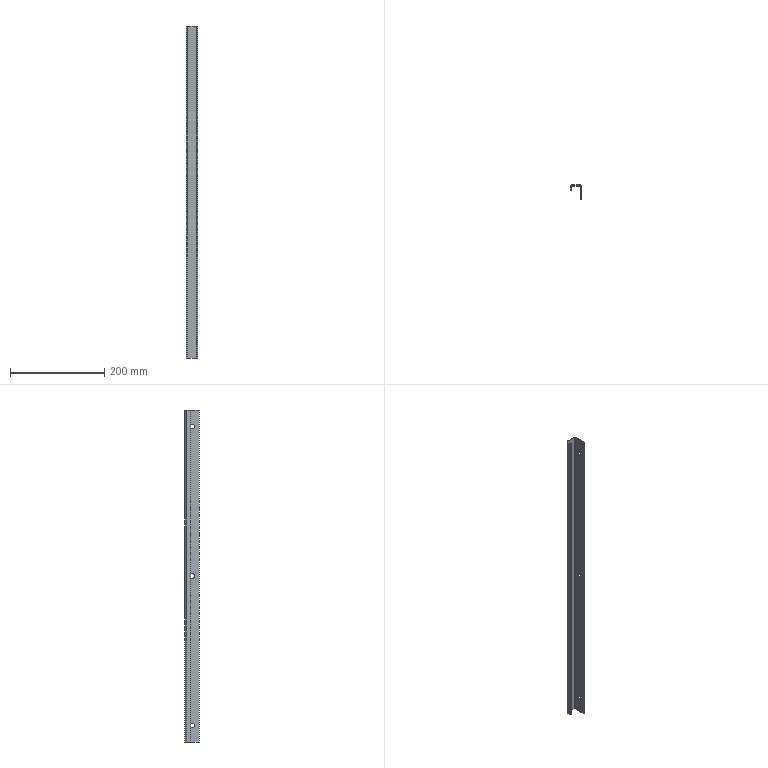Part | STEP file | 750078266 | 1 solid | 20 faces | box 25 x 30 x 704 mm | volume 84559 mm3 | cylinder 10 | plane 10 | commonest cylinder face diameters 10.5 x6 4 x2 8 x2
STEP:
#1=CARTESIAN_POINT('',(-2.,15.,322.25));
#2=VERTEX_POINT('',#1);
#3=CARTESIAN_POINT('',(-2.,15.,311.75));
#4=VERTEX_POINT('',#3);
#5=CARTESIAN_POINT('',(-2.,15.,317.));
#6=DIRECTION('',(1.,0.,0.));
#7=DIRECTION('',(0.,0.,-1.));
#8=AXIS2_PLACEMENT_3D('',#5,#6,#7);
#9=CIRCLE('',#8,5.25);
#10=EDGE_CURVE('',#2,#4,#9,.T.);
#11=ORIENTED_EDGE('',*,*,#10,.F.);
#12=CARTESIAN_POINT('',(0.,15.,322.25));
#13=VERTEX_POINT('',#12);
#14=CARTESIAN_POINT('',(-2.,15.,322.25));
#15=DIRECTION('',(1.,0.,0.));
#16=VECTOR('',#15,1000.);
#17=LINE('',#14,#16);
#18=EDGE_CURVE('',#2,#13,#17,.T.);
#19=ORIENTED_EDGE('',*,*,#18,.T.);
#20=CARTESIAN_POINT('',(0.,15.,311.75));
#21=VERTEX_POINT('',#20);
#22=CARTESIAN_POINT('',(0.,15.,317.));
#23=DIRECTION('',(-1.,0.,0.));
#24=DIRECTION('',(0.,0.,-1.));
#25=AXIS2_PLACEMENT_3D('',#22,#23,#24);
#26=CIRCLE('',#25,5.25);
#27=EDGE_CURVE('',#21,#13,#26,.T.);
#28=ORIENTED_EDGE('',*,*,#27,.F.);
#29=CARTESIAN_POINT('',(-2.,15.,311.75));
#30=DIRECTION('',(1.,0.,0.));
#31=VECTOR('',#30,1000.);
#32=LINE('',#29,#31);
#33=EDGE_CURVE('',#4,#21,#32,.T.);
#34=ORIENTED_EDGE('',*,*,#33,.F.);
#35=EDGE_LOOP('',(#11,#19,#28,#34));
#36=FACE_OUTER_BOUND('',#35,.T.);
#37=CARTESIAN_POINT('',(-2.,15.,317.));
#38=DIRECTION('',(1.,0.,0.));
#39=DIRECTION('',(0.,0.,-1.));
#40=AXIS2_PLACEMENT_3D('',#37,#38,#39);
#41=CYLINDRICAL_SURFACE('',#40,5.25);
#42=ADVANCED_FACE('',(#36),#41,.F.);
#43=CARTESIAN_POINT('',(-2.,15.,5.25));
#44=VERTEX_POINT('',#43);
#45=CARTESIAN_POINT('',(-2.,15.,-5.25));
#46=VERTEX_POINT('',#45);
#47=CARTESIAN_POINT('',(-2.,15.,0.));
#48=DIRECTION('',(1.,0.,0.));
#49=DIRECTION('',(0.,0.,-1.));
#50=AXIS2_PLACEMENT_3D('',#47,#48,#49);
#51=CIRCLE('',#50,5.25);
#52=EDGE_CURVE('',#44,#46,#51,.T.);
#53=ORIENTED_EDGE('',*,*,#52,.F.);
#54=CARTESIAN_POINT('',(0.,15.,5.25));
#55=VERTEX_POINT('',#54);
#56=CARTESIAN_POINT('',(-2.,15.,5.25));
#57=DIRECTION('',(1.,0.,0.));
#58=VECTOR('',#57,1000.);
#59=LINE('',#56,#58);
#60=EDGE_CURVE('',#44,#55,#59,.T.);
#61=ORIENTED_EDGE('',*,*,#60,.T.);
#62=CARTESIAN_POINT('',(0.,15.,-5.25));
#63=VERTEX_POINT('',#62);
#64=CARTESIAN_POINT('',(0.,15.,0.));
#65=DIRECTION('',(-1.,0.,0.));
#66=DIRECTION('',(0.,0.,-1.));
#67=AXIS2_PLACEMENT_3D('',#64,#65,#66);
#68=CIRCLE('',#67,5.25);
#69=EDGE_CURVE('',#63,#55,#68,.T.);
#70=ORIENTED_EDGE('',*,*,#69,.F.);
#71=CARTESIAN_POINT('',(-2.,15.,-5.25));
#72=DIRECTION('',(1.,0.,0.));
#73=VECTOR('',#72,1000.);
#74=LINE('',#71,#73);
#75=EDGE_CURVE('',#46,#63,#74,.T.);
#76=ORIENTED_EDGE('',*,*,#75,.F.);
#77=EDGE_LOOP('',(#53,#61,#70,#76));
#78=FACE_OUTER_BOUND('',#77,.T.);
#79=CARTESIAN_POINT('',(-2.,15.,0.));
#80=DIRECTION('',(1.,0.,0.));
#81=DIRECTION('',(0.,0.,-1.));
#82=AXIS2_PLACEMENT_3D('',#79,#80,#81);
#83=CYLINDRICAL_SURFACE('',#82,5.25);
#84=ADVANCED_FACE('',(#78),#83,.F.);
#85=CARTESIAN_POINT('',(-2.,15.,-311.75));
#86=VERTEX_POINT('',#85);
#87=CARTESIAN_POINT('',(-2.,15.,-322.25));
#88=VERTEX_POINT('',#87);
#89=CARTESIAN_POINT('',(-2.,15.,-317.));
#90=DIRECTION('',(1.,0.,0.));
#91=DIRECTION('',(0.,0.,-1.));
#92=AXIS2_PLACEMENT_3D('',#89,#90,#91);
#93=CIRCLE('',#92,5.25);
#94=EDGE_CURVE('',#86,#88,#93,.T.);
#95=ORIENTED_EDGE('',*,*,#94,.F.);
#96=CARTESIAN_POINT('',(0.,15.,-311.75));
#97=VERTEX_POINT('',#96);
#98=CARTESIAN_POINT('',(-2.,15.,-311.75));
#99=DIRECTION('',(1.,0.,0.));
#100=VECTOR('',#99,1000.);
#101=LINE('',#98,#100);
#102=EDGE_CURVE('',#86,#97,#101,.T.);
#103=ORIENTED_EDGE('',*,*,#102,.T.);
#104=CARTESIAN_POINT('',(0.,15.,-322.25));
#105=VERTEX_POINT('',#104);
#106=CARTESIAN_POINT('',(0.,15.,-317.));
#107=DIRECTION('',(-1.,0.,0.));
#108=DIRECTION('',(0.,0.,-1.));
#109=AXIS2_PLACEMENT_3D('',#106,#107,#108);
#110=CIRCLE('',#109,5.25);
#111=EDGE_CURVE('',#105,#97,#110,.T.);
#112=ORIENTED_EDGE('',*,*,#111,.F.);
#113=CARTESIAN_POINT('',(-2.,15.,-322.25));
#114=DIRECTION('',(1.,0.,0.));
#115=VECTOR('',#114,1000.);
#116=LINE('',#113,#115);
#117=EDGE_CURVE('',#88,#105,#116,.T.);
#118=ORIENTED_EDGE('',*,*,#117,.F.);
#119=EDGE_LOOP('',(#95,#103,#112,#118));
#120=FACE_OUTER_BOUND('',#119,.T.);
#121=CARTESIAN_POINT('',(-2.,15.,-317.));
#122=DIRECTION('',(1.,0.,0.));
#123=DIRECTION('',(0.,0.,-1.));
#124=AXIS2_PLACEMENT_3D('',#121,#122,#123);
#125=CYLINDRICAL_SURFACE('',#124,5.25);
#126=ADVANCED_FACE('',(#120),#125,.F.);
#127=CARTESIAN_POINT('',(0.,26.,352.));
#128=VERTEX_POINT('',#127);
#129=CARTESIAN_POINT('',(0.,0.,352.));
#130=VERTEX_POINT('',#129);
#131=CARTESIAN_POINT('',(0.,30.,352.));
#132=DIRECTION('',(0.,-1.,0.));
#133=VECTOR('',#132,1000.);
#134=LINE('',#131,#133);
#135=EDGE_CURVE('',#128,#130,#134,.T.);
#136=ORIENTED_EDGE('',*,*,#135,.T.);
#137=CARTESIAN_POINT('',(0.,0.,-352.));
#138=VERTEX_POINT('',#137);
#139=CARTESIAN_POINT('',(0.,0.,352.));
#140=DIRECTION('',(0.,0.,-1.));
#141=VECTOR('',#140,1000.);
#142=LINE('',#139,#141);
#143=EDGE_CURVE('',#130,#138,#142,.T.);
#144=ORIENTED_EDGE('',*,*,#143,.T.);
#145=CARTESIAN_POINT('',(0.,26.,-352.));
#146=VERTEX_POINT('',#145);
#147=CARTESIAN_POINT('',(0.,30.,-352.));
#148=DIRECTION('',(0.,1.,0.));
#149=VECTOR('',#148,1000.);
#150=LINE('',#147,#149);
#151=EDGE_CURVE('',#138,#146,#150,.T.);
#152=ORIENTED_EDGE('',*,*,#151,.T.);
#153=CARTESIAN_POINT('',(0.,26.,352.));
#154=DIRECTION('',(0.,0.,1.));
#155=VECTOR('',#154,1000.);
#156=LINE('',#153,#155);
#157=EDGE_CURVE('',#146,#128,#156,.T.);
#158=ORIENTED_EDGE('',*,*,#157,.T.);
#159=EDGE_LOOP('',(#136,#144,#152,#158));
#160=FACE_OUTER_BOUND('',#159,.T.);
#161=ORIENTED_EDGE('',*,*,#27,.T.);
#162=CARTESIAN_POINT('',(0.,15.,317.));
#163=DIRECTION('',(-1.,0.,0.));
#164=DIRECTION('',(0.,0.,-1.));
#165=AXIS2_PLACEMENT_3D('',#162,#163,#164);
#166=CIRCLE('',#165,5.25);
#167=EDGE_CURVE('',#13,#21,#166,.T.);
#168=ORIENTED_EDGE('',*,*,#167,.T.);
#169=EDGE_LOOP('',(#161,#168));
#170=FACE_BOUND('',#169,.T.);
#171=ORIENTED_EDGE('',*,*,#69,.T.);
#172=CARTESIAN_POINT('',(0.,15.,0.));
#173=DIRECTION('',(-1.,0.,0.));
#174=DIRECTION('',(0.,0.,-1.));
#175=AXIS2_PLACEMENT_3D('',#172,#173,#174);
#176=CIRCLE('',#175,5.25);
#177=EDGE_CURVE('',#55,#63,#176,.T.);
#178=ORIENTED_EDGE('',*,*,#177,.T.);
#179=EDGE_LOOP('',(#171,#178));
#180=FACE_BOUND('',#179,.T.);
#181=ORIENTED_EDGE('',*,*,#111,.T.);
#182=CARTESIAN_POINT('',(0.,15.,-317.));
#183=DIRECTION('',(-1.,0.,0.));
#184=DIRECTION('',(0.,0.,-1.));
#185=AXIS2_PLACEMENT_3D('',#182,#183,#184);
#186=CIRCLE('',#185,5.25);
#187=EDGE_CURVE('',#97,#105,#186,.T.);
#188=ORIENTED_EDGE('',*,*,#187,.T.);
#189=EDGE_LOOP('',(#181,#188));
#190=FACE_BOUND('',#189,.T.);
#191=CARTESIAN_POINT('',(0.,30.,352.));
#192=DIRECTION('',(1.,0.,0.));
#193=DIRECTION('',(0.,0.,-1.));
#194=AXIS2_PLACEMENT_3D('',#191,#192,#193);
#195=PLANE('',#194);
#196=ADVANCED_FACE('',(#160,#170,#180,#190),#195,.T.);
#197=CARTESIAN_POINT('',(-2.,0.,-352.));
#198=VERTEX_POINT('',#197);
#199=CARTESIAN_POINT('',(0.,0.,-352.));
#200=DIRECTION('',(1.,0.,0.));
#201=VECTOR('',#200,1000.);
#202=LINE('',#199,#201);
#203=EDGE_CURVE('',#198,#138,#202,.T.);
#204=ORIENTED_EDGE('',*,*,#203,.T.);
#205=ORIENTED_EDGE('',*,*,#143,.F.);
#206=CARTESIAN_POINT('',(-2.,0.,352.));
#207=VERTEX_POINT('',#206);
#208=CARTESIAN_POINT('',(0.,0.,352.));
#209=DIRECTION('',(-1.,0.,0.));
#210=VECTOR('',#209,1000.);
#211=LINE('',#208,#210);
#212=EDGE_CURVE('',#130,#207,#211,.T.);
#213=ORIENTED_EDGE('',*,*,#212,.T.);
#214=CARTESIAN_POINT('',(-2.,0.,352.));
#215=DIRECTION('',(0.,0.,-1.));
#216=VECTOR('',#215,1000.);
#217=LINE('',#214,#216);
#218=EDGE_CURVE('',#207,#198,#217,.T.);
#219=ORIENTED_EDGE('',*,*,#218,.T.);
#220=EDGE_LOOP('',(#204,#205,#213,#219));
#221=FACE_OUTER_BOUND('',#220,.T.);
#222=CARTESIAN_POINT('',(0.,0.,352.));
#223=DIRECTION('',(0.,-1.,0.));
#224=DIRECTION('',(0.,0.,-1.));
#225=AXIS2_PLACEMENT_3D('',#222,#223,#224);
#226=PLANE('',#225);
#227=ADVANCED_FACE('',(#221),#226,.T.);
#228=CARTESIAN_POINT('',(-2.,26.,352.));
#229=VERTEX_POINT('',#228);
#230=CARTESIAN_POINT('',(-2.,30.,352.));
#231=DIRECTION('',(0.,-1.,0.));
#232=VECTOR('',#231,1000.);
#233=LINE('',#230,#232);
#234=EDGE_CURVE('',#229,#207,#233,.T.);
#235=ORIENTED_EDGE('',*,*,#234,.T.);
#236=ORIENTED_EDGE('',*,*,#212,.F.);
#237=ORIENTED_EDGE('',*,*,#135,.F.);
#238=CARTESIAN_POINT('',(-4.,30.,352.));
#239=VERTEX_POINT('',#238);
#240=CARTESIAN_POINT('',(-4.,26.,352.));
#241=DIRECTION('',(0.,0.,1.));
#242=DIRECTION('',(-1.,0.,0.));
#243=AXIS2_PLACEMENT_3D('',#240,#241,#242);
#244=CIRCLE('',#243,4.);
#245=EDGE_CURVE('',#128,#239,#244,.T.);
#246=ORIENTED_EDGE('',*,*,#245,.T.);
#247=CARTESIAN_POINT('',(-21.,30.,352.));
#248=VERTEX_POINT('',#247);
#249=CARTESIAN_POINT('',(0.,30.,352.));
#250=DIRECTION('',(-1.,0.,0.));
#251=VECTOR('',#250,1000.);
#252=LINE('',#249,#251);
#253=EDGE_CURVE('',#239,#248,#252,.T.);
#254=ORIENTED_EDGE('',*,*,#253,.T.);
#255=CARTESIAN_POINT('',(-25.,26.,352.));
#256=VERTEX_POINT('',#255);
#257=CARTESIAN_POINT('',(-21.,26.,352.));
#258=DIRECTION('',(0.,0.,1.));
#259=DIRECTION('',(-1.,0.,0.));
#260=AXIS2_PLACEMENT_3D('',#257,#258,#259);
#261=CIRCLE('',#260,4.);
#262=EDGE_CURVE('',#248,#256,#261,.T.);
#263=ORIENTED_EDGE('',*,*,#262,.T.);
#264=CARTESIAN_POINT('',(-25.,18.,352.));
#265=VERTEX_POINT('',#264);
#266=CARTESIAN_POINT('',(-25.,30.,352.));
#267=DIRECTION('',(0.,-1.,0.));
#268=VECTOR('',#267,1000.);
#269=LINE('',#266,#268);
#270=EDGE_CURVE('',#256,#265,#269,.T.);
#271=ORIENTED_EDGE('',*,*,#270,.T.);
#272=CARTESIAN_POINT('',(-23.,18.,352.));
#273=VERTEX_POINT('',#272);
#274=CARTESIAN_POINT('',(0.,18.,352.));
#275=DIRECTION('',(1.,0.,0.));
#276=VECTOR('',#275,1000.);
#277=LINE('',#274,#276);
#278=EDGE_CURVE('',#265,#273,#277,.T.);
#279=ORIENTED_EDGE('',*,*,#278,.T.);
#280=CARTESIAN_POINT('',(-23.,26.,352.));
#281=VERTEX_POINT('',#280);
#282=CARTESIAN_POINT('',(-23.,30.,352.));
#283=DIRECTION('',(0.,1.,0.));
#284=VECTOR('',#283,1000.);
#285=LINE('',#282,#284);
#286=EDGE_CURVE('',#273,#281,#285,.T.);
#287=ORIENTED_EDGE('',*,*,#286,.T.);
#288=CARTESIAN_POINT('',(-21.,28.,352.));
#289=VERTEX_POINT('',#288);
#290=CARTESIAN_POINT('',(-21.,26.,352.));
#291=DIRECTION('',(0.,0.,-1.));
#292=DIRECTION('',(-1.,0.,0.));
#293=AXIS2_PLACEMENT_3D('',#290,#291,#292);
#294=CIRCLE('',#293,2.);
#295=EDGE_CURVE('',#281,#289,#294,.T.);
#296=ORIENTED_EDGE('',*,*,#295,.T.);
#297=CARTESIAN_POINT('',(-4.,28.,352.));
#298=VERTEX_POINT('',#297);
#299=CARTESIAN_POINT('',(0.,28.,352.));
#300=DIRECTION('',(1.,0.,0.));
#301=VECTOR('',#300,1000.);
#302=LINE('',#299,#301);
#303=EDGE_CURVE('',#289,#298,#302,.T.);
#304=ORIENTED_EDGE('',*,*,#303,.T.);
#305=CARTESIAN_POINT('',(-4.,26.,352.));
#306=DIRECTION('',(0.,0.,-1.));
#307=DIRECTION('',(-1.,0.,0.));
#308=AXIS2_PLACEMENT_3D('',#305,#306,#307);
#309=CIRCLE('',#308,2.);
#310=EDGE_CURVE('',#298,#229,#309,.T.);
#311=ORIENTED_EDGE('',*,*,#310,.T.);
#312=EDGE_LOOP('',(#235,#236,#237,#246,#254,#263,#271,#279,#287,#296,#304,#311));
#313=FACE_OUTER_BOUND('',#312,.T.);
#314=CARTESIAN_POINT('',(0.,30.,352.));
#315=DIRECTION('',(0.,0.,1.));
#316=DIRECTION('',(1.,0.,0.));
#317=AXIS2_PLACEMENT_3D('',#314,#315,#316);
#318=PLANE('',#317);
#319=ADVANCED_FACE('',(#313),#318,.T.);
#320=ORIENTED_EDGE('',*,*,#245,.F.);
#321=ORIENTED_EDGE('',*,*,#157,.F.);
#322=CARTESIAN_POINT('',(-4.,30.,-352.));
#323=VERTEX_POINT('',#322);
#324=CARTESIAN_POINT('',(-4.,26.,-352.));
#325=DIRECTION('',(0.,0.,1.));
#326=DIRECTION('',(-1.,0.,0.));
#327=AXIS2_PLACEMENT_3D('',#324,#325,#326);
#328=CIRCLE('',#327,4.);
#329=EDGE_CURVE('',#146,#323,#328,.T.);
#330=ORIENTED_EDGE('',*,*,#329,.T.);
#331=CARTESIAN_POINT('',(-4.,30.,352.));
#332=DIRECTION('',(0.,0.,1.));
#333=VECTOR('',#332,1000.);
#334=LINE('',#331,#333);
#335=EDGE_CURVE('',#323,#239,#334,.T.);
#336=ORIENTED_EDGE('',*,*,#335,.T.);
#337=EDGE_LOOP('',(#320,#321,#330,#336));
#338=FACE_OUTER_BOUND('',#337,.T.);
#339=CARTESIAN_POINT('',(-4.,26.,352.));
#340=DIRECTION('',(0.,0.,-1.));
#341=DIRECTION('',(-1.,0.,0.));
#342=AXIS2_PLACEMENT_3D('',#339,#340,#341);
#343=CYLINDRICAL_SURFACE('',#342,4.);
#344=ADVANCED_FACE('',(#338),#343,.T.);
#345=CARTESIAN_POINT('',(-21.,30.,-352.));
#346=VERTEX_POINT('',#345);
#347=CARTESIAN_POINT('',(-25.,26.,-352.));
#348=VERTEX_POINT('',#347);
#349=CARTESIAN_POINT('',(-21.,26.,-352.));
#350=DIRECTION('',(0.,0.,1.));
#351=DIRECTION('',(-1.,0.,0.));
#352=AXIS2_PLACEMENT_3D('',#349,#350,#351);
#353=CIRCLE('',#352,4.);
#354=EDGE_CURVE('',#346,#348,#353,.T.);
#355=ORIENTED_EDGE('',*,*,#354,.F.);
#356=CARTESIAN_POINT('',(-25.,30.,-352.));
#357=DIRECTION('',(-1.,0.,0.));
#358=VECTOR('',#357,1000.);
#359=LINE('',#356,#358);
#360=EDGE_CURVE('',#323,#346,#359,.T.);
#361=ORIENTED_EDGE('',*,*,#360,.F.);
#362=ORIENTED_EDGE('',*,*,#329,.F.);
#363=ORIENTED_EDGE('',*,*,#151,.F.);
#364=ORIENTED_EDGE('',*,*,#203,.F.);
#365=CARTESIAN_POINT('',(-2.,26.,-352.));
#366=VERTEX_POINT('',#365);
#367=CARTESIAN_POINT('',(-2.,18.,-352.));
#368=DIRECTION('',(0.,-1.,0.));
#369=VECTOR('',#368,1000.);
#370=LINE('',#367,#369);
#371=EDGE_CURVE('',#366,#198,#370,.T.);
#372=ORIENTED_EDGE('',*,*,#371,.F.);
#373=CARTESIAN_POINT('',(-4.,28.,-352.));
#374=VERTEX_POINT('',#373);
#375=CARTESIAN_POINT('',(-4.,26.,-352.));
#376=DIRECTION('',(0.,0.,-1.));
#377=DIRECTION('',(-1.,0.,0.));
#378=AXIS2_PLACEMENT_3D('',#375,#376,#377);
#379=CIRCLE('',#378,2.);
#380=EDGE_CURVE('',#374,#366,#379,.T.);
#381=ORIENTED_EDGE('',*,*,#380,.F.);
#382=CARTESIAN_POINT('',(-21.,28.,-352.));
#383=VERTEX_POINT('',#382);
#384=CARTESIAN_POINT('',(-25.,28.,-352.));
#385=DIRECTION('',(1.,0.,0.));
#386=VECTOR('',#385,1000.);
#387=LINE('',#384,#386);
#388=EDGE_CURVE('',#383,#374,#387,.T.);
#389=ORIENTED_EDGE('',*,*,#388,.F.);
#390=CARTESIAN_POINT('',(-23.,26.,-352.));
#391=VERTEX_POINT('',#390);
#392=CARTESIAN_POINT('',(-21.,26.,-352.));
#393=DIRECTION('',(0.,0.,-1.));
#394=DIRECTION('',(-1.,0.,0.));
#395=AXIS2_PLACEMENT_3D('',#392,#393,#394);
#396=CIRCLE('',#395,2.);
#397=EDGE_CURVE('',#391,#383,#396,.T.);
#398=ORIENTED_EDGE('',*,*,#397,.F.);
#399=CARTESIAN_POINT('',(-23.,18.,-352.));
#400=VERTEX_POINT('',#399);
#401=CARTESIAN_POINT('',(-23.,18.,-352.));
#402=DIRECTION('',(0.,1.,0.));
#403=VECTOR('',#402,1000.);
#404=LINE('',#401,#403);
#405=EDGE_CURVE('',#400,#391,#404,.T.);
#406=ORIENTED_EDGE('',*,*,#405,.F.);
#407=CARTESIAN_POINT('',(-25.,18.,-352.));
#408=VERTEX_POINT('',#407);
#409=CARTESIAN_POINT('',(-25.,18.,-352.));
#410=DIRECTION('',(1.,0.,0.));
#411=VECTOR('',#410,1000.);
#412=LINE('',#409,#411);
#413=EDGE_CURVE('',#408,#400,#412,.T.);
#414=ORIENTED_EDGE('',*,*,#413,.F.);
#415=CARTESIAN_POINT('',(-25.,18.,-352.));
#416=DIRECTION('',(0.,-1.,0.));
#417=VECTOR('',#416,1000.);
#418=LINE('',#415,#417);
#419=EDGE_CURVE('',#348,#408,#418,.T.);
#420=ORIENTED_EDGE('',*,*,#419,.F.);
#421=EDGE_LOOP('',(#355,#361,#362,#363,#364,#372,#381,#389,#398,#406,#414,#420));
#422=FACE_OUTER_BOUND('',#421,.T.);
#423=CARTESIAN_POINT('',(-25.,18.,-352.));
#424=DIRECTION('',(0.,0.,1.));
#425=DIRECTION('',(1.,0.,0.));
#426=AXIS2_PLACEMENT_3D('',#423,#424,#425);
#427=PLANE('',#426);
#428=ADVANCED_FACE('',(#422),#427,.F.);
#429=ORIENTED_EDGE('',*,*,#18,.F.);
#430=CARTESIAN_POINT('',(-2.,15.,317.));
#431=DIRECTION('',(1.,0.,0.));
#432=DIRECTION('',(0.,0.,-1.));
#433=AXIS2_PLACEMENT_3D('',#430,#431,#432);
#434=CIRCLE('',#433,5.25);
#435=EDGE_CURVE('',#4,#2,#434,.T.);
#436=ORIENTED_EDGE('',*,*,#435,.F.);
#437=ORIENTED_EDGE('',*,*,#33,.T.);
#438=ORIENTED_EDGE('',*,*,#167,.F.);
#439=EDGE_LOOP('',(#429,#436,#437,#438));
#440=FACE_OUTER_BOUND('',#439,.T.);
#441=CARTESIAN_POINT('',(-2.,15.,317.));
#442=DIRECTION('',(1.,0.,0.));
#443=DIRECTION('',(0.,0.,-1.));
#444=AXIS2_PLACEMENT_3D('',#441,#442,#443);
#445=CYLINDRICAL_SURFACE('',#444,5.25);
#446=ADVANCED_FACE('',(#440),#445,.F.);
#447=ORIENTED_EDGE('',*,*,#60,.F.);
#448=CARTESIAN_POINT('',(-2.,15.,0.));
#449=DIRECTION('',(1.,0.,0.));
#450=DIRECTION('',(0.,0.,-1.));
#451=AXIS2_PLACEMENT_3D('',#448,#449,#450);
#452=CIRCLE('',#451,5.25);
#453=EDGE_CURVE('',#46,#44,#452,.T.);
#454=ORIENTED_EDGE('',*,*,#453,.F.);
#455=ORIENTED_EDGE('',*,*,#75,.T.);
#456=ORIENTED_EDGE('',*,*,#177,.F.);
#457=EDGE_LOOP('',(#447,#454,#455,#456));
#458=FACE_OUTER_BOUND('',#457,.T.);
#459=CARTESIAN_POINT('',(-2.,15.,0.));
#460=DIRECTION('',(1.,0.,0.));
#461=DIRECTION('',(0.,0.,-1.));
#462=AXIS2_PLACEMENT_3D('',#459,#460,#461);
#463=CYLINDRICAL_SURFACE('',#462,5.25);
#464=ADVANCED_FACE('',(#458),#463,.F.);
#465=ORIENTED_EDGE('',*,*,#102,.F.);
#466=CARTESIAN_POINT('',(-2.,15.,-317.));
#467=DIRECTION('',(1.,0.,0.));
#468=DIRECTION('',(0.,0.,-1.));
#469=AXIS2_PLACEMENT_3D('',#466,#467,#468);
#470=CIRCLE('',#469,5.25);
#471=EDGE_CURVE('',#88,#86,#470,.T.);
#472=ORIENTED_EDGE('',*,*,#471,.F.);
#473=ORIENTED_EDGE('',*,*,#117,.T.);
#474=ORIENTED_EDGE('',*,*,#187,.F.);
#475=EDGE_LOOP('',(#465,#472,#473,#474));
#476=FACE_OUTER_BOUND('',#475,.T.);
#477=CARTESIAN_POINT('',(-2.,15.,-317.));
#478=DIRECTION('',(1.,0.,0.));
#479=DIRECTION('',(0.,0.,-1.));
#480=AXIS2_PLACEMENT_3D('',#477,#478,#479);
#481=CYLINDRICAL_SURFACE('',#480,5.25);
#482=ADVANCED_FACE('',(#476),#481,.F.);
#483=ORIENTED_EDGE('',*,*,#218,.F.);
#484=ORIENTED_EDGE('',*,*,#234,.F.);
#485=CARTESIAN_POINT('',(-2.,26.,352.));
#486=DIRECTION('',(0.,0.,1.));
#487=VECTOR('',#486,1000.);
#488=LINE('',#485,#487);
#489=EDGE_CURVE('',#366,#229,#488,.T.);
#490=ORIENTED_EDGE('',*,*,#489,.F.);
#491=ORIENTED_EDGE('',*,*,#371,.T.);
#492=EDGE_LOOP('',(#483,#484,#490,#491));
#493=FACE_OUTER_BOUND('',#492,.T.);
#494=ORIENTED_EDGE('',*,*,#435,.T.);
#495=ORIENTED_EDGE('',*,*,#10,.T.);
#496=EDGE_LOOP('',(#494,#495));
#497=FACE_BOUND('',#496,.T.);
#498=ORIENTED_EDGE('',*,*,#453,.T.);
#499=ORIENTED_EDGE('',*,*,#52,.T.);
#500=EDGE_LOOP('',(#498,#499));
#501=FACE_BOUND('',#500,.T.);
#502=ORIENTED_EDGE('',*,*,#471,.T.);
#503=ORIENTED_EDGE('',*,*,#94,.T.);
#504=EDGE_LOOP('',(#502,#503));
#505=FACE_BOUND('',#504,.T.);
#506=CARTESIAN_POINT('',(-2.,30.,352.));
#507=DIRECTION('',(1.,0.,0.));
#508=DIRECTION('',(0.,0.,-1.));
#509=AXIS2_PLACEMENT_3D('',#506,#507,#508);
#510=PLANE('',#509);
#511=ADVANCED_FACE('',(#493,#497,#501,#505),#510,.F.);
#512=ORIENTED_EDGE('',*,*,#489,.T.);
#513=ORIENTED_EDGE('',*,*,#310,.F.);
#514=CARTESIAN_POINT('',(-4.,28.,352.));
#515=DIRECTION('',(0.,0.,1.));
#516=VECTOR('',#515,1000.);
#517=LINE('',#514,#516);
#518=EDGE_CURVE('',#374,#298,#517,.T.);
#519=ORIENTED_EDGE('',*,*,#518,.F.);
#520=ORIENTED_EDGE('',*,*,#380,.T.);
#521=EDGE_LOOP('',(#512,#513,#519,#520));
#522=FACE_OUTER_BOUND('',#521,.T.);
#523=CARTESIAN_POINT('',(-4.,26.,352.));
#524=DIRECTION('',(0.,0.,-1.));
#525=DIRECTION('',(-1.,0.,0.));
#526=AXIS2_PLACEMENT_3D('',#523,#524,#525);
#527=CYLINDRICAL_SURFACE('',#526,2.);
#528=ADVANCED_FACE('',(#522),#527,.F.);
#529=ORIENTED_EDGE('',*,*,#518,.T.);
#530=ORIENTED_EDGE('',*,*,#303,.F.);
#531=CARTESIAN_POINT('',(-21.,28.,352.));
#532=DIRECTION('',(0.,0.,1.));
#533=VECTOR('',#532,1000.);
#534=LINE('',#531,#533);
#535=EDGE_CURVE('',#383,#289,#534,.T.);
#536=ORIENTED_EDGE('',*,*,#535,.F.);
#537=ORIENTED_EDGE('',*,*,#388,.T.);
#538=EDGE_LOOP('',(#529,#530,#536,#537));
#539=FACE_OUTER_BOUND('',#538,.T.);
#540=CARTESIAN_POINT('',(-25.,28.,352.));
#541=DIRECTION('',(0.,1.,0.));
#542=DIRECTION('',(0.,0.,1.));
#543=AXIS2_PLACEMENT_3D('',#540,#541,#542);
#544=PLANE('',#543);
#545=ADVANCED_FACE('',(#539),#544,.F.);
#546=ORIENTED_EDGE('',*,*,#535,.T.);
#547=ORIENTED_EDGE('',*,*,#295,.F.);
#548=CARTESIAN_POINT('',(-23.,26.,352.));
#549=DIRECTION('',(0.,0.,1.));
#550=VECTOR('',#549,1000.);
#551=LINE('',#548,#550);
#552=EDGE_CURVE('',#391,#281,#551,.T.);
#553=ORIENTED_EDGE('',*,*,#552,.F.);
#554=ORIENTED_EDGE('',*,*,#397,.T.);
#555=EDGE_LOOP('',(#546,#547,#553,#554));
#556=FACE_OUTER_BOUND('',#555,.T.);
#557=CARTESIAN_POINT('',(-21.,26.,352.));
#558=DIRECTION('',(0.,0.,-1.));
#559=DIRECTION('',(-1.,0.,0.));
#560=AXIS2_PLACEMENT_3D('',#557,#558,#559);
#561=CYLINDRICAL_SURFACE('',#560,2.);
#562=ADVANCED_FACE('',(#556),#561,.F.);
#563=ORIENTED_EDGE('',*,*,#552,.T.);
#564=ORIENTED_EDGE('',*,*,#286,.F.);
#565=CARTESIAN_POINT('',(-23.,18.,352.));
#566=DIRECTION('',(0.,0.,1.));
#567=VECTOR('',#566,1000.);
#568=LINE('',#565,#567);
#569=EDGE_CURVE('',#400,#273,#568,.T.);
#570=ORIENTED_EDGE('',*,*,#569,.F.);
#571=ORIENTED_EDGE('',*,*,#405,.T.);
#572=EDGE_LOOP('',(#563,#564,#570,#571));
#573=FACE_OUTER_BOUND('',#572,.T.);
#574=CARTESIAN_POINT('',(-23.,18.,352.));
#575=DIRECTION('',(-1.,0.,0.));
#576=DIRECTION('',(0.,0.,1.));
#577=AXIS2_PLACEMENT_3D('',#574,#575,#576);
#578=PLANE('',#577);
#579=ADVANCED_FACE('',(#573),#578,.F.);
#580=ORIENTED_EDGE('',*,*,#278,.F.);
#581=CARTESIAN_POINT('',(-25.,18.,352.));
#582=DIRECTION('',(0.,0.,1.));
#583=VECTOR('',#582,1000.);
#584=LINE('',#581,#583);
#585=EDGE_CURVE('',#408,#265,#584,.T.);
#586=ORIENTED_EDGE('',*,*,#585,.F.);
#587=ORIENTED_EDGE('',*,*,#413,.T.);
#588=ORIENTED_EDGE('',*,*,#569,.T.);
#589=EDGE_LOOP('',(#580,#586,#587,#588));
#590=FACE_OUTER_BOUND('',#589,.T.);
#591=CARTESIAN_POINT('',(-25.,18.,352.));
#592=DIRECTION('',(0.,1.,0.));
#593=DIRECTION('',(0.,0.,1.));
#594=AXIS2_PLACEMENT_3D('',#591,#592,#593);
#595=PLANE('',#594);
#596=ADVANCED_FACE('',(#590),#595,.F.);
#597=ORIENTED_EDGE('',*,*,#270,.F.);
#598=CARTESIAN_POINT('',(-25.,26.,352.));
#599=DIRECTION('',(0.,0.,-1.));
#600=VECTOR('',#599,1000.);
#601=LINE('',#598,#600);
#602=EDGE_CURVE('',#256,#348,#601,.T.);
#603=ORIENTED_EDGE('',*,*,#602,.T.);
#604=ORIENTED_EDGE('',*,*,#419,.T.);
#605=ORIENTED_EDGE('',*,*,#585,.T.);
#606=EDGE_LOOP('',(#597,#603,#604,#605));
#607=FACE_OUTER_BOUND('',#606,.T.);
#608=CARTESIAN_POINT('',(-25.,18.,352.));
#609=DIRECTION('',(-1.,0.,0.));
#610=DIRECTION('',(0.,0.,1.));
#611=AXIS2_PLACEMENT_3D('',#608,#609,#610);
#612=PLANE('',#611);
#613=ADVANCED_FACE('',(#607),#612,.T.);
#614=ORIENTED_EDGE('',*,*,#262,.F.);
#615=CARTESIAN_POINT('',(-21.,30.,352.));
#616=DIRECTION('',(0.,0.,-1.));
#617=VECTOR('',#616,1000.);
#618=LINE('',#615,#617);
#619=EDGE_CURVE('',#248,#346,#618,.T.);
#620=ORIENTED_EDGE('',*,*,#619,.T.);
#621=ORIENTED_EDGE('',*,*,#354,.T.);
#622=ORIENTED_EDGE('',*,*,#602,.F.);
#623=EDGE_LOOP('',(#614,#620,#621,#622));
#624=FACE_OUTER_BOUND('',#623,.T.);
#625=CARTESIAN_POINT('',(-21.,26.,352.));
#626=DIRECTION('',(0.,0.,-1.));
#627=DIRECTION('',(-1.,0.,0.));
#628=AXIS2_PLACEMENT_3D('',#625,#626,#627);
#629=CYLINDRICAL_SURFACE('',#628,4.);
#630=ADVANCED_FACE('',(#624),#629,.T.);
#631=ORIENTED_EDGE('',*,*,#253,.F.);
#632=ORIENTED_EDGE('',*,*,#335,.F.);
#633=ORIENTED_EDGE('',*,*,#360,.T.);
#634=ORIENTED_EDGE('',*,*,#619,.F.);
#635=EDGE_LOOP('',(#631,#632,#633,#634));
#636=FACE_OUTER_BOUND('',#635,.T.);
#637=CARTESIAN_POINT('',(-25.,30.,352.));
#638=DIRECTION('',(0.,1.,0.));
#639=DIRECTION('',(0.,0.,1.));
#640=AXIS2_PLACEMENT_3D('',#637,#638,#639);
#641=PLANE('',#640);
#642=ADVANCED_FACE('',(#636),#641,.T.);
#643=CLOSED_SHELL('',(#42,#84,#126,#196,#227,#319,#344,#428,#446,#464,#482,#511,#528,#545,#562,#579,#596,#613,#630,#642));
#644=MANIFOLD_SOLID_BREP('',#643);
#645=CARTESIAN_POINT('',(0.,0.,0.));
#646=DIRECTION('',(0.,0.,1.));
#647=DIRECTION('',(1.,0.,0.));
#648=AXIS2_PLACEMENT_3D('',#645,#646,#647);
#649=(LENGTH_UNIT()NAMED_UNIT(*)SI_UNIT(.MILLI.,.METRE.));
#650=UNCERTAINTY_MEASURE_WITH_UNIT(LENGTH_MEASURE(0.00001),#649,'','');
#651=(NAMED_UNIT(*)PLANE_ANGLE_UNIT()SI_UNIT($,.RADIAN.));
#652=(NAMED_UNIT(*)SI_UNIT($,.STERADIAN.)SOLID_ANGLE_UNIT());
#653=(GEOMETRIC_REPRESENTATION_CONTEXT(3)GLOBAL_UNCERTAINTY_ASSIGNED_CONTEXT((#650))GLOBAL_UNIT_ASSIGNED_CONTEXT((#649,#651,#652))REPRESENTATION_CONTEXT('',''));
#654=ADVANCED_BREP_SHAPE_REPRESENTATION('',(#644,#648),#653);